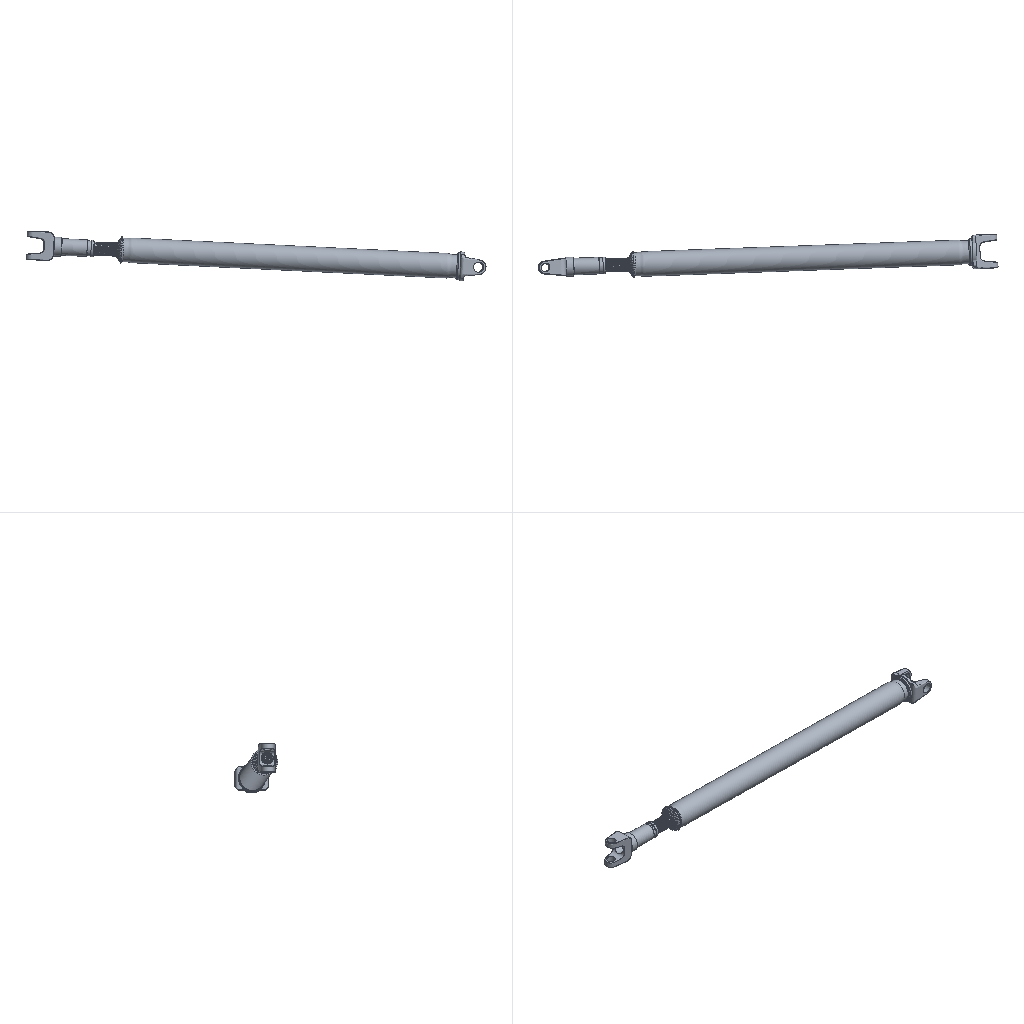Simulation study | nastran
Set-up summary:
category,name,step,type,value,unit,region
solver,nx_nastran
units,not stated in the deck,,not stated
analysis,deck,,static,static
analysis,solution,,SOL,101
load_step,SUBCASE 2,2,SUBCASE,SPC=2 LOAD=3
load_step,requested,,,1
mesh,nodes,,,78810
mesh,elements,,,190757
element_type,CBEAM,,unverified,2
element_type,CHEXA,,solid,14946
element_type,CPENTA,,solid,664
element_type,CQUAD4,,shell,29350
element_type,CTETRA,,solid,145789
element_type,CTRIA3,,shell,8
load,nodal force total,,FX,0.0,model units
load,nodal force total,,FY,0.0,model units
load,nodal force total,,FZ,0.0,model units
load,load commands in deck,,count,1
bc,support commands in deck,,count,1065
check,setup vs results,,match,"every grid point's frame and coordinates and every element id; grid points of CBEAM, CHEXA, CPENTA, CQUAD4, CTETRA, CTRIA3 elements"
Nastran input file, long lists of numbers shortened:
$$------------------------------------------------------------------------------$
$$                                                                              $
$$ NASTRAN Input Deck Generated by HyperMesh Version  :11.0.0.4                 $
$$ Generated using HyperMesh-Nastran Template Version : 11.0.0.47
$$                                                                              $
$$   Template:  general                                                         $
$$                                                                              $
$$------------------------------------------------------------------------------$
$$------------------------------------------------------------------------------$
$$                      Executive Control Cards                                 $
$$------------------------------------------------------------------------------$
SOL 101
$$------------------------------------------------------------------------------$
$$                      Case Control Cards                                      $
$$------------------------------------------------------------------------------$
SET 2 = 2476004 THRU 2502367
$HMSET        2        2 "2D"
$HMSETTYPE       2 "regular"
SET 3 = 7051 THRU 62103,88428 THRU 179163,
        1247402 THRU 1253317,1256926 THRU 1258666,
        1258668 THRU 1258718,1258720 THRU 1258744,
        1258746 THRU 1258770,1258772 THRU 1258796,
        1258798 THRU 1258822,1258824 THRU 1258848,
        1258850 THRU 1258874,1258876 THRU 1258926,
        1258928 THRU 1259242,1259332 THRU 1261639,
        2282969 THRU 2288002
$HMSET        3        2 "3D"
$HMSETTYPE       3 "regular"
  DISPLACEMENT = ALL
  STRAIN = ALL
  STRESS = ALL
$
$HMNAME LOADSTEP               2"torsion"
SUBCASE       2
  LABEL= torsion
  SPC =        2
  LOAD =        3
  STRESS = 3
$$------------------------------------------------------------------------------$
$$                      Bulk Data Cards                                         $
$$------------------------------------------------------------------------------$
BEGIN BULK
PARAM,AUTOSPC,YES
PARAM,POST,-1
$HMNAME SYSTCOL                1"auto1"
$HWCOLOR SYSTCOL               1       3
$$
$$  SYSTEM Data
$$
CORD2R         1        1229.955-4.75192-230.4771235.19 -4.75192-130.614+
+       1329.741-.828432-235.708
CORD2R         2        1293.315-2.43806-233.5351299.369-2.43806-133.718+
+       1393.0561.448555-239.584
$HMNAME SYSTCOL                2"systemcollector1"
$HWCOLOR SYSTCOL               2       4
CORD2R         3        1114.16 -8.99358-224.8341108.925-8.99358-324.697+
+       1110.24290.92943-224.629
$$
$$  GRID Data
$$
GRID           1        1174.03717.26392-252.005
GRID           2        1174.11 15.26483-252.009
$ (78808 more lines like these left out)
$$
$$  SPOINT Data
$$
$$
$$  CBEAM Elements
$$
CBEAM    2582172       4  498701  4987061.0     0.0     0.0             +
+              1
CBEAM    2582173       4  498705  4987021.0     0.0     0.0             +
+              1
$
$HMMOVE       34
$        2582172THRU     2582173
$
$$
$$------------------------------------------------------------------------------$
$$             Group Definitions                                                $
$$------------------------------------------------------------------------------$
$$
$$ RBE2 Elements - Multiple dependent nodes
$$
RBE2     2417732  498701  123456  291538  291540  291584  291585  291728+
+         291731  291732  291735  291736  291739  291740  291743  291744+
+         291747  291748  291751  291752  291755  291756  291759  291760+
+         291763  291764  291832  291926  291937  291940  291942  291944+
+         291946  291947  291949  291951  291953  291955  291973  291974+
+         291975  291976  291977  291978  291979  291980  291981  292320+
+         292321  292322  292323  292324  292325  292326  292327  292328+
+         292329  292330  292331  292332  292333  292334  292335  292336+
+         292337  292447  292448  292450  292464  292465  292466  292467+
+         292468  292469  292470  292471  292472  292473  292474  292475+
+         292476  292477  292478  292479  292480  292481  292518  292519+
+         292520  292521  292522  292523  292524  498553  498554  498555+
+         498556  498557  498558  498559  498560  498561  498562  498563+
+         498564  498565  498566  498567  498568  498569  498570  498571+
+         498572  498573  498574  498575  498576  498577  498578  498579+
+         498580  498581  498582  498583  498584  498585  498586  498587+
+         498588  498589  498590  498591  498592  498593  498594  498595+
+         498596  498597  498598  498599  498600  498601  498602  498603+
+         498604  498605  498606  498607  498608  498609  498610  498611+
+         498612  498613  498614  498615  498616  498617  498618  498619+
+         498620  498621  498622  498623  498624  498625  498626  498627+
+         498628  498629  498630  498631  498632  498633  498634  498635+
+         498636  498637  498638  498639  498640  498641  498642  498643+
+         498644  498645  498646  498647  498648  498649  498650  498651+
+         498652  498653  498654  498655  498656
RBE2     2417733  498702  123456  296642  302624  302625  302628  302629+
+         302632  302633  302636  302637  302640  302641  302644  302645+
+         302648  302649  302652  302653  302656  302657  302660  302661+
+         302664  302665  302668  302669  302672  302673  302676  302677+
+         302680  302681  302684  302685  302688  302689  302692  302693+
+         302696  302697  302700  302701  302704  302705  302708  302709+
+         302712  302713  302716  302717  302720  302721  302724  302725+
+         302728  302730  302732  302734  302736  302738  302740  302742+
+         302744  302746  302748  302750  302752  302754  302756  302758+
+         302760  302762  302764  302766  302768  302770  302772  302774+
+         302776  302778  304865  304867  304869  304871  304873  304875+
+         304877  304879  304881  304883  304885  304887  304889  304891+
+         304893  304895  304897  304899  304901  304903  304905  304907+
+         304909  304911  304913  304920  304921  304924  304925  304928+
+         304929  304932  304933  304936  304937  304940  304941  304944+
+         304945  304948  304949  304952  304953  304956  304967  304970+
+         304971  304974  304975  304978  304979  304982  304983  304986+
+         304987  304990  304991  304994  304995  304998  304999  305002+
+         305003  305008  305009  305012  305013  305016  305017  305020+
+         305021  305024  305025  305028  305029  498529  498530
RBE2     2421920  498705  123456  282536  282537  282538  282539  282672+
+         282673  282760  282761  282848  282849  282916  282980  282981+
+         283048  283112  283113  283180  283244  283245  283312  283356+
+         283400  283464  283465  283552  283553  283620  283664  283708+
+         283752  283816  283817  283884  283928  283972  284016  284060+
+         284104  284148  284212  284213  284280  284324  284368  284412+
+         284456  284500  284544  284608  284609  284676  284720  284764+
+         284808  284852  284896  284940  285004  285005  285072  285116+
+         285160  285204  285248  285292  285356  285357  285424  285468+
+         285512  285556  285600  285644  285708  285709  285776  285820+
+         285864  285908  285952  285996  286040  286104  286105  286172+
+         286216  286260  286304  286348  286392  286436  286500  286501+
+         286568  286612  286656  286700  286744  286788  286852  286853+
+         286920  286964  287008  290080  290114  290182  290218  290265+
+         290322  290362  290393  290455  290499  290548  290632  290676+
+         290712  290772  290781  290871  290936  290982  291030  291078+
+         291149  291150  291153  291244  291545  291546  291699  291895+
+         292255  292406  292430  292737  292804  292805  292869  292937+
+         293024  293025  293119  293120  293257  293262  294269  294313+
+         294357  294425  294489  294533  294577  294621  294665  294709+
+         294777  294841  294885  294929  294973  295017  295061  295105+
+         295173  295237  295281  295325  295369  295413  295457  295501+
+         295569  295633  295677  295721  295765  295809  295853  295921+
+         295985  296029  296073  296117  296161  296205  296273  296337+
+         296381  296425  296469  296513  296557
RBE2     2421921  498706  123456  300253  300274  300277  303716  303717+
+         303718  303719  303720  303721  303722  303723  303724  303725+
+         303726  303727  303728  303729  303730  303731  303732  303733+
+         303734  303735  303736  303737  303738  303739  303740  303741+
+         303742  303743  303744  303745  303746  303747  303748  303749+
+         303750  303751  303752  303753  303754  303755  303756  303757+
+         303758  303759  303760  303761  303762  303763  303764  303765+
+         303766  303767  303768  303769  303770  303771  303772  303773+
+         303774  303775  303776  303777  303778  303779  303780  303781+
+         303782  303783  303784  303785  303786  303787  303788  303789+
+         303790  303791  303792  303793  303835  303836  303837  303838+
+         303839  303840  303841  303842  303843  303844  303845  303846+
+         303847  303848  303849  303850  303851  303852  303853  303854+
+         303855  303856  303857  303858  303859  303862  303863  303864+
+         303865  303866  303867  303868  303869  303870  303871  303872+
+         303873  303874  303875  303876  303877  303878  303879  303880+
+         303881  303882  303883  303884  303885  303886  303887  303888+
+         303889  303890  303891  303892  303893  303894  303895  303896+
+         303897  303898  303899  303900  303901  303902  303903  303904+
+         303905  303906  303907  303908  303909  303910  303911
RBE2     2641893  525195  123456     889     890     891     892     893+
+            894     895     896     897     898     899     900     901+
+            902     903     904     905     906     907     908     909+
+            910     911     912     913     914     915     916     917+
+            918     919     920     921     922     923     924     925+
+            926     927     928    2664    2665    2666    2667    2668+
+           2669    2670    2671    2672    2673    2674    2675    2676+
+           2677    2678    2679    2680    2681    2682    2683    2684+
+           2685    2686    2687    2688    2689    2690    2691    2692+
+           2693    2694    2695    2696    2697    2698    2699    2700+
+           2701    2702    2703    2704    2705    2706    2707    2708+
+           2709    2710    2711    2712    2713    2714    2715    2716+
+           2717    2718    2719    2720    2721    2722    2723    2724+
+           2725    2726    2727    2728    2729    2730    2731    2732+
+           2733    2734    2735    2736    2737    2738    2739    2740+
+           2741    2742    2743    2744    2745    2746    2747    2748+
+           2749    2750    2751    2752    2753    2754    2755    2756+
+           2757    2758    2759    2760    2761    2762    2763    2764+
+           2765    2766    2767    2768    2769    2770    2771    2772+
+           2773    2774    2775    2776    2777    2778    2779    2780+
+           2781    2782    2783    2784    2785    2786    2787    2788+
+           2789    2790    2791    2792    2793    2794    2795    2796+
+           2797    2798    2799    2800    2801    2802    2803    2804+
+           2805    2806    2807    2808    2809    2810    2811    2812+
+           2813    2814    2815    2816    2817    2818    2819    2820+
+           2821    2822    2823    2824    2825    2826    2827    2828+
+           2829    2830    2831    2832    2833    2834    2835    2836+
+           2837    2838    2839    2840    2841    2842    2843    2844+
+           2845    2846    2847    2848    2849    2850    2851    2852+
+           2853    2854    2855    2856    2857    2858    2859    2860+
+           2861    2862    2863    2864    2865    2866    2867    2868+
+           2869    2870    2871    2872    2873    2874    2875    2876+
+           2877    2878    2879    2880    2881    2882    2883    2884+
+           2885    2886    2887    2888    2889    2890    2891    2892+
+           2893    2894    2895    2896    2897    2898    2899    2900+
+           2901    2902    2903    2904    2905    2906    2907    2908+
+           2909    2910    2911    2912    2913    2914    2915    2916+
+           2917    2918    2919    2920    2921    2922    2923    2924+
+           2925    2926    2927    2928    2929    2930    2931    2932+
+           2933    2934    2935    2936    2937    2938    2939    2940+
+           2941    2942    2943    2944    2945    2946    2947    2948+
+           2949    2950    2951    2952    2953    2954    2955    2956+
+           2957    2958    2959    2960    2961    2962    2963    2964+
+           2965    2966    2967    2968    2969    2970    2971    2972+
+           2973    2974    2975    2976    2977    2978    2979    2980+
+           2981    2982    2983    2984    2985    2986    2987    2988+
+           2989    2990    2991    2992    2993    2994    2995    2996+
+           2997    2998    2999    3000    3001    3002    3003    3004+
+           3005    3006    3007    3008    3009    3010    3011    3012+
+           3013    3014    3015    3016    3017    3018    3019    3020+
+           3021    3022    3023    3887    3888    3889    3890    3891+
+           3892    3893    3894    3895    3896    3897    3898    3899+
+           3900    3901    3902    3903    3904    3905    3906    3907+
+           3908    3909    3910    3911    3912    3913    3914    3915+
+           3916    3917    3918    3919    3920    3921    3922    3923+
+           3924    3925    3926    5763    5764    5765    5766    5767+
+           5768    5769    5770    5771    5772    5773    5774    5775+
+           5776    5777    5778    5779    5780    5781    5782    5783+
+           5784    5785    5786    5787    5788    5789    5790    5791+
+           5792    5793    5794    5795    5796    5797    5798    5799+
+           5800    5801    5802    5803    5804    5805    5806    5807+
+           5808    5809    5810    5811    5812    5813    5814    5815+
+           5816    5817    5818    5819    5820    5821    5822    5823+
+           5824    5825    5826    5827    5828    5829    5830    5831+
+           5832    5833    5834    5835    5836    5837    5838    5839+
+           5840    5841    5842    5843    5844    5845    5846    5847+
+           5848    5849    5850    5851    5852    5853    5854    5855+
+           5856    5857    5858    5859    5860    5861    5862    5863+
+           5864    5865    5866    5867    5868    5869    5870    5871+
+           5872    5873    5874    5875    5876    5877    5878    5879+
+           5880    5881    5882    5883    5884    5885    5886    5887+
+           5888    5889    5890    5891    5892    5893    5894    5895+
+           5896    5897    5898    5899    5900    5901    5902    5903+
+           5904    5905    5906    5907    5908    5909    5910    5911+
+           5912    5913    5914    5915    5916    5917    5918    5919+
+           5920    5921    5922    5923    5924    5925    5926    5927+
+           5928    5929    5930    5931    5932    5933    5934    5935+
+           5936    5937    5938    5939    5940    5941    5942    5943+
+           5944    5945    5946    5947    5948    5949    5950    5951+
+           5952    5953    5954    5955    5956    5957    5958    5959+
+           5960    5961    5962    5963    5964    5965    5966    5967+
+           5968    5969    5970    5971    5972    5973    5974    5975+
+           5976    5977    5978    5979    5980    5981    5982    5983+
+           5984    5985    5986    5987    5988    5989    5990    5991+
+           5992    5993    5994    5995    5996    5997    5998    5999+
+           6000    6001    6002    6003    6004    6005    6006    6007+
+           6008    6009    6010    6011    6012    6013    6014    6015+
+           6016    6017    6018    6019    6020    6021    6022    6023+
+           6024    6025    6026    6027    6028    6029    6030    6031+
+           6032    6033    6034    6035    6036    6037    6038    6039+
+           6040    6041    6042    6043    6044    6045    6046    6047+
+           6048    6049    6050    6051    6052    6053    6054    6055+
+           6056    6057    6058    6059    6060    6061    6062    6063+
+           6064    6065    6066    6067    6068    6069    6070    6071+
+           6072    6073    6074    6075    6076    6077    6078    6079+
+           6080    6081    6082    6083    6084    6085    6086    6087+
+           6088    6089    6090    6091    6092    6093    6094    6095+
+           6096    6097    6098    6099    6100    6101    6102    6103+
+           6104    6105    6106    6107    6108    6109    6110    6111+
+           6112    6113    6114    6115    6116    6117    6118    6119+
+           6120    6121    6122
RBE2     2664129  525197  123456   24038   24039   24040   24041   24042+
+          24043   24044   24045   24046   24047   24048   24049   24050+
+          24051   24052   24053   24054   24055   24056   24057   24058+
+          24059   24060   24061   24062   24063   24064   24065   24066+
+          24067   24068   24069   24070   24071   24072   24073   24074+
+          24075   24076   24077   24078   24079   24080   24081   24082+
+          24083   24084   24085   24086   24087   24088   24089   24090+
+          24091   24092   24093   24094   24095   24096   24097   24098+
+          24099   24100   24101   24102   24103   24104   24105   24106+
+          24107   24108   24109   24110   24111   24112   24113   24114+
+          24115   24116   24117   24118   24119   24120   24121   24122+
+          24123   24124   24125   24126   24127   24128   24129   24130+
+          24131   24132   24133   24134   24135   24136   24137   24138+
+          24139   24140   24141   24142   24143   24144   24145   24146+
+          24147   24148   24149   24150   24151   24152   24153   24154+
+          24155   24156   24157   24158   24159   24160   24161   24162+
+          24163   24164   24165   24166   24167   24168   24169   24170+
+          24171   24172   24173   24174   24175   24176   24177   24178+
+          24179   24180   24181   24182   24183   24184   24185   24186+
+          24187   24188   24189   24190   24191   24192   24193   24194+
+          24195   24196   24197   24198   24199   24683   24686   24688+
+          24690   24692   24694   24696   24698   24700   24702   24704+
+          24706   24708   24710   24712   24714   24716   24718   24719+
+          24721   24723   24725   24727   24729   24731   24733   24735+
+          26414   26416   26418   26420   26422   26423   26439   26445+
+          26466   26469   26470   26471   26474   26476   26479   26480+
+          26482   26486   26487   26488   26489   26492   26495   26496+
+          26497   26500   26914   26919   26920   26921   26922   26923+
+          26924   26925   26926   26927   26928   26929   26930   26931+
+          26932   26933   26934   26935   26936   26937   26938   26939+
+          26940   26941   26942   26943   26944   26945   26946   26947+
+          26948   26949   26950   26951   26952   26953   26954   26955+
+          26956   26957   26958   26959   26960   26961   26962   26963+
+          26964   26965   26966   26967   26968   26969   26970   26971+
+          26972   26973   26974   26975   26976   26977   26978   26979+
+          26980   26981   26982   26983   26984   26985   26986   26987+
+          26988   26989   26990   26991   26992   26993   26994   26995+
+          26996   26997   26998   26999   27000   27001   27011   27012+
+          27013   27014   27015   27016   27017   27018   27019   27020+
+          27021   27022   27023   27024   27025   27026   27027   27028+
+          27029   27030   27031   27032   27033   27034   27035   27036+
+          27037   27038   27039   27040   27041   27042   27043   27044+
+          27045   27046   27047   27048   27049   27050   27051   27052+
+          27053   27054   27055   27056   27057   27058   27062   27063+
+          27065   27066   27067   27068   27069   27070   27071   27072+
+          27073   27074   27075   27076   27077   27078   27079   27080+
+          27081   27082   27083   27084   27085   27086   29537   29538+
+          29539   29540   29541   29542   29543   29544   29545   29546+
+          29547   29548   29549   29550   29557   29558   29559   29560+
+          29561   29562   29565   29566   29567   29568   29569   29570+
+          29574   29575   29576   29577   29578   29579   29597   29598+
+          29599   29600   29601   29602   29603   29604   29605   29606+
+          29607   29608   29609   29610   29611   29612   29613   29614+
+          29615   29616   29617   29618   29619   29620   29621   29622+
+          29623   29624   29625   29626   29627   29628   29629   29630+
+          29631   29632   29633   29634   29635   29636   29637   29638+
+          29639   29640   29641   29642   29643   29644   29650   29651+
+          29652   29653   29654   29655   29656   29657   29658   29659+
+          29660   29675   29676   29677   29678   29701   29702   29703+
+          29704   29705   29706   29707   29708   29709   29710   29711+
+          29712   29713   29714   29715   29716   29717   29718   29719+
+          29720   29721   29722   29723   29724   29725   29726   29727+
+          29728   29729   29730   29731   29732   29733   29734   29735+
+          29736   29737   29738   29739   29740   29741   29742   29743+
+          29744   29745   29746   29747   29748   29749   29750   29751+
+          29752   29753   29754   29756   30084   30086   30088   30092+
+          30100   30101   30103   30139   30141   30149   30150   30151+
+          30153   30154   30157   30159   30160   30161   30171   30181+
+          30188   30191   30192   30194   30201   30655   31210   31213+
+          31215   31217   31219   31221   31222   31240   31246   31267+
+          31270   31271   31272   31275   31277   31280   31281   31283+
+          31287   31288   31289   31290   31295   31299   31300   31303+
+          31734   31739   31740   31741   31742   31743   31744   31745+
+          31746   31747   31748   31749   31750   31751   31752   31753+
+          31754   31755   31756   31757   31758   31759   31760   31761+
+          31762   31763   31764   31765   31766   31767   31768   31769+
+          31770   31771   31772   31773   31774   31775   31776   31777+
+          31778   31779   31780   31781   31782   31783   31784   31785+
+          31786   31787   31788   31789   31790   31791   31792   31793+
+          31794   31795   31796   31800   31801   31802   31803   31804+
+          31805   31806   31807   31808   31809   31810   31811   31812+
+          31813   31814   31815   31816   31817   31818   31819   31820+
+          31821   31822   31823   31832   31833   31834   31835   31836+
+          31837   31838   31839   31840   31841   31842   31843   31844+
+          31845   31846   31847   31848   31849   31850   31851   31852+
+          31853   31854   31855   31856   31857   31858   31859   31860+
+          31861   31862   31863   31864   31865   31866   31867   31868+
+          31869   31870   31871   31872   31873   31874   31875   31876+
+          31877   31878   31879   31880   31881   31882   31883   31884+
+          31885   31886   31887   31888   31889   31890   31891   31892+
+          31893   31894   31895   31896   31897   31898   31899   31900+
+          31901   31902   31903  498746  498747  498748  498749  498750+
+         498793  498794  498795  498796  498797  498798  498799  498800+
+         498801  498802  498803  498804  498805  498806  498807  498808+
+         498809  498810  498811  498812  498813  498814  498815  498816+
+         498817  498818  498819  498820  498821  498822  498823  498824+
+         498825  498826  498827  498828  498829  498830  498831  498832+
+         498833  498834  498835  498837  498838  498839  498840  498842+
+         498843  498844  498845  498847  498848  498849  498850  498851+
+         498852  498853  498854  498856  498858  498860  498861  498862+
+         498863  498864  498865  498866  498867  498868  498869  498870+
+         498872  498874  498875  498878  498879  498880  498881  498882+
+         498883  498884  498885  498887  498888  498889  498890  498891+
+         498892  498893  498894  498895  498897  498899  498900  498903+
+         498904  498905  498906  498907  498908  498909  498910  498911+
+         498912  498913  498914  498915  498917  498919  498920  498923+
+         498924  498925  498926  498927  498928  498929  498930  498932+
+         498933  498934  498935  498937  498938  498939  498940  498941+
+         498942  498943  498944  498945  498947  498949  498950  498953+
+         498954  498955  498956  498957  498958  498959  498960  498961+
+         498962  498963  498964  498965  498967  498969  498970  498973+
+         498974  498975  498976  498977  498978  498979  498980  498982+
+         498983  498984  498985  498986  498987  498988  498989  498990+
+         498992  498994  498995  498998  498999  499000  499001  499002+
+         499003  499004  499005  499006  499007  499008  499009  499010+
+         499012  499014  499015  499018  499019  499020  499021  499022+
+         499023  499024  499025  499026  499027  499028  499029  499030+
+         499031  499032  499033  499034  499035  499036  499037  499038+
+         499039  499040  499041  499042  499043  499044  499045  499046+
+         499047  499048  499049  499050  499051  499052  499053  499054+
+         499055  499056  499057  499058  499059  499060  499061  499062+
+         499063  499103  499104  499105  499106  499108  499109  499110+
+         499111  499113  499114  499115  499116  499117  499118  499119+
+         499120  499122  499124  499126  499127  499128  499129  499130+
+         499131  499132  499133  499134  499135  499136  499138  499140+
+         499141  499144  499145  499146  499147  499148  499149  499150+
+         499151  499153  499154  499155  499156  499157  499158  499159+
+         499160  499161  499163  499165  499166  499169  499170  499171+
+         499172  499173  499174  499175  499176  499177  499178  499179+
+         499180  499181  499183  499185  499186  499189  499190  499191+
+         499192  499193  499194  499195  499196  499198  499199  499200+
+         499201  499203  499204  499205  499206  499207  499208  499209+
+         499210  499211  499213  499215  499216  499219  499220  499221+
+         499222  499223  499224  499225  499226  499227  499228  499229+
+         499230  499231  499233  499235  499236  499239  499240  499241+
+         499242  499243  499244  499245  499246  499248  499249  499250+
+         499251  499252  499253  499254  499255  499256  499258  499260+
+         499261  499264  499265  499266  499267  499268  499269  499270+
+         499271  499272  499273  499274  499275  499276  499278  499280+
+         499281  499284  499285  499286  499287  499288  499289  499290+
+         499291
RBE2     2682332  525198  123456       1       2       3       4       5+
+              6       7       8       9      10      11      12      13+
+             14      53      70      86      91      92      97      98+
+            116     121     122     127     128     204     205     206+
+            207     208     209     210     211     212     213     214+
+            215     216     217     218     219     220     221     222+
+            223     224     225     226     227     228     229     230+
+            231     232     233     234     235     236     237     238+
+            239     240     241     242     243     244     245     246+
+            247     248     249     250     251     252     253     254+
+            255     256     257     258     259     260     261     262+
+            263     264     265     266     267     268     269     270+
+            271     272     273     274     275     276     277     278+
+            279     280     281     282     283     284     285     286+
+            287     288     289     290     291     292     293     294+
+            295     296     297     298     299     300     301     302+
+            303     304     305     306     307     308     309     310+
+            311     312     313     314     315     316     317     318+
+            319     320     321     322     323     324     325     326+
+            327     328     329     330     331     332     333     334+
+            335     336     337     338     339     340     341     342+
+            343     344     345     346     347     348     349     350+
+            351     352     353     354     355     356     357     358+
+            359     360     361     362     363     364     365     366+
+            367     368     369     370     371     372     373     374+
+            375     376     377     378     379     380     381     382+
+            383     384     385     386     387     388     389     390+
+            391     392     393     394     395     396     397     398+
+            399     400     401     402     403     404     405     406+
+            407     408     409     410     411     412     413     414+
+            415     416     417     418     419     420     421     422+
+            423     424     425     426     427     428     429     430+
+            431     432     433     434     435     436     437     438+
+            439     440     441     442     443     444     445     446+
+            447     448     449     450     451     452     453     454+
+            455     456     457     458     459     460     461     462+
+            463     464     465     466     467     468     469     470+
+            471     472     473     474     475     476     477     478+
+            479     480     481     482     483     484     485     486+
+            487     488     489     490     491     492     493     494+
+            495     496     497     498     499     500     501     502+
+            503     504     505     506     507     508     509     510+
+            511     512     513     514     515     516     517     518+
+            519     520     521     522     523     524     525     526+
+            527     528     529     530     531     532     533     534+
+            535     536     537     538     539     540     541     542+
+            543     544     545     546     547     548     549     550+
+            551     552     553     554     555     556     557     558+
+            559     560     561     562     563     564     565     566+
+            567     568     569     570     571     572     573     574+
+            575     576     577     578     579     580     581     582+
+            583     584     585     586     587     588     589     590+
+            591     592     593     594     595     596     597     598+
+            599     600     601     602     603     604     605     606+
+            607     608     609     610     611     612     613     614+
+            615     616     617     618     619     620     621     622+
+            623     624     625     626     627     628     629     630+
+            631     632     633     634     635     636     637     638+
+            639     640     641     642     654     743     757     762+
+            763     768     769     792     797     798     803     804+
+           1343    1344    1433    1447    1452    1453    1458    1459+
+           1482    1487    1488    1493    1494    1534    1551    1567+
+           1572    1573    1578    1579    1597    1602    1603    1608+
+           1609  300414  300416  300417  300419  300420  300422  300423+
+         300425  300426  300428  300429  300431  300432  300434  300435+
+         300437  300438  300440  300441  300443  300444  300446  300447+
+         300449  300450  300452  300453  300455  300456  300458  300459+
+         300461  300462  300464  300465  300467  300468  300470  300471+
+         300473  300474  300476  300477  300479  300480  300482  300483+
+         300485  300486  300488  300489  300491  300544  300545  300546+
+         300547  300548  300549  300550  300551  300552  300553  300554+
+         300555  300556  300557  300558  300559  300560  300561  300562+
+         300563  300564  300565  300566  300567  300568  300569  300570+
+         300571  300572  300573  300574  300575  300576  300577  300578+
+         300579  300580  300581  300582  300583  300584  300585  300586+
+         300587  300588  300589  300590  300591  300592  300593  300594+
+         300595  307113  307114  307115  307116  307117  307118  307119+
+         307120  307121  307122  307123  307124  307125  307126  307127+
+         307128  307129  307130  307131  307132  307133  307134  307135+
+         307136  307137  307139  307142  307143  307144  307145  307146+
+         307147  307148  307149  307150  307151  307152  307153  307154+
+         307155  307156  307157  307158  307159  307160  307161  307162+
+         307163  307164  307165  307229  307231  307232  307234  307235+
+         307237  307238  307240  307241  307243  307244  307246  307247+
+         307249  307250  307252  307253  307255  307256  307258  307259+
+         307261  307262  307264  307265  307267  307268  307270  307271+
+         307273  307274  307276  307277  307279  307280  307282  307283+
+         307285  307286  307288  307289  307291  307292  307294  307295+
+         307297  307298  307300  307301  307303  498509  498550  498551+
+         498552
$
$HMMOVE       24
$        2417732THRU     2417733 2421920THRU     2421921
$
$
$HMMOVE       54
$        2641893 2664129 2682332
$
$
$  RBE3 Elements
$
RBE3     2690425          527713  123456.2075213     123  524945.7866865+
+            123  524944.0045832     123  5249490.001209     123  524951
RBE3     2690426          527714  1234561.0-5        123  292235  292236+
+       .6874827     123  292588.3125173     123  292367
$ (348 more lines like these left out)
$
$HMMOVE       55
$        2690425THRU     2690430 2690432THRU     2690434 2690436THRU     2690438
$        2690440THRU     2690442 2690444THRU     2690446 2690448THRU     2690450
$        2690452THRU     2690454 2690456THRU     2690458 2690460THRU     2690462
$        2690464THRU     2690466 2690468THRU     2690470 2690472THRU     2690474
$        2690476THRU     2690478 2690480THRU     2690482 2690484THRU     2690486
$        2690488THRU     2690490 2690492THRU     2690494 2690496THRU     2690498
$        2690500THRU     2690502 2690504THRU     2690506 2690508THRU     2690510
$        2690512THRU     2690514 2690516THRU     2690518 2690520THRU     2690522
$        2690524THRU     2690526 2690528THRU     2690530 2690532THRU     2690534
$        2690536THRU     2690538 2690540THRU     2690542 2690544THRU     2690546
$        2690548THRU     2690550 2690552THRU     2690554 2690556THRU     2690558
$        2690560THRU     2690562 2690564THRU     2690566 2690568THRU     2690570
$        2690572THRU     2690574 2690576THRU     2690578 2690580THRU     2690582
$        2690584THRU     2690586 2690588THRU     2690590 2690592THRU     2690594
$        2690596THRU     2690598
$
$$
$$  CTRIA3 Data
$$
CTRIA3   2686784       6  292326  292328  292480
CTRIA3   2686785       6  293484  293483  293482
CTRIA3   2686786       6  293457  293456  293455
CTRIA3   2686787       6  291974  291732  291940
CTRIA3   2686788       6  498642  498648  498644
CTRIA3   2686789       6  498595  498590  498592
CTRIA3   2686790       6  289148  289149  289147
CTRIA3   2686791       6  289175  289176  289174
$
$HMMOVE       57
$        2686784THRU     2686791
$
$
$  CQUAD4 Elements
$
CQUAD4   2476004       5  498852  498854  498856  498851
CQUAD4   2476005       5  498851  498856  498847  498848
$ (29348 more lines like these left out)
$
$HMMOVE       48
$        2476004THRU     2502367
$
$
$HMMOVE       57
$        2686792THRU     2689777
$
$
$  CHEXA Elements: First Order
$
CHEXA    1256926       1  296579  296580  296582  296581  300310  300313+
+         300312  300311
CHEXA    1256927       1  300310  300313  300312  300311  300314  300317+
+         300316  300315
$ (29888 more lines like these left out)
$
$HMMOVE       18
$        1256926THRU     1257497 1257524THRU     1258511 1258538THRU     1258666
$        1258668THRU     1258718 1258720THRU     1258744 1258746THRU     1258770
$ (31 more lines like these left out)
CTETRA     10206       1    8149    8032    2891    8163
CTETRA     10207       1    7673    2872    2974    2970
$ (145787 more lines like these left out)
$
$  CPENTA Elements 6-noded
$
CPENTA   1257498       1  498536  296619  498535  301480  301429  301377
CPENTA   1257499       1  301480  301429  301377  301481  301431  301379
$ (662 more lines like these left out)
$
$HMMOVE        9
$          10206THRU       10322   11200THRU       12082    9227THRU        9343
$          10323THRU       11088   12083THRU       12160   12250THRU       12288
$ (192 more lines like these left out)
PSHELL         5       11.8            1               1
$
$HMNAME PROP                   6"face" 4
$HWCOLOR PROP                  6      45
PSHELL         6       20.1            2               2
$
$
$
$
$
$$
$$  PSOLID Data
$
$HMNAME PROP                   1"steel" 5
$HWCOLOR PROP                  1       6
PSOLID         1       1
$
$HMNAME PROP                   7"seam" 5
$HWCOLOR PROP                  7      45
PSOLID         7       1
$$
$$  PBEAM Data
$
$HMNAME PROP                   4"beam" 3
$HWCOLOR PROP                  4       5
$HMBEAMSEC PBEAMASSOC          4       7
PBEAM          4       11256.637125663.7125663.70.0     251327.4
+
+
+                                       0.0     0.0
$$--------------------------------------------------------------
$$ HYPERMESH TAGS
$$--------------------------------------------------------------
$$BEGIN TAGS
$$END TAGS
$$
$$  MAT1 Data
$
$HMNAME MAT                    1"steel" "MAT1"
$HWCOLOR MAT                   1       3
MAT1           1210000.0        0.28    7.8-9
$
$HMNAME MAT                    2"face" "MAT1"
$HWCOLOR MAT                   2       3
MAT1           22.1             0.3     7.8-20
$$
$$
$$
$$------------------------------------------------------------------------------$
$ (32 more lines like these left out)
SPC            2   23075  1234560.0
SPC            2   23076  1234560.0
SPC            2   23077  1234560.0
SPC            2   23078  1234560.0
$ (1061 more lines like these left out)
$
$$
$$  MOMENT Data
$$
MOMENT         3  525195       31.0     2.581-111305000.4.366-11
ENDDATA
$$CONNECTORS_XML_INFO_START
$$<?xml version="1.0" encoding="ISO-8859-1" ?>
$$<MasterConnectorFile>
$$<!--                                                                         -->
$ (259 more lines like these left out)
Results summary:
result,analysis,,,static
result,last_loadstep,,,1
result,primary field,,,displacements
result,max displacement,,,1.876,model units